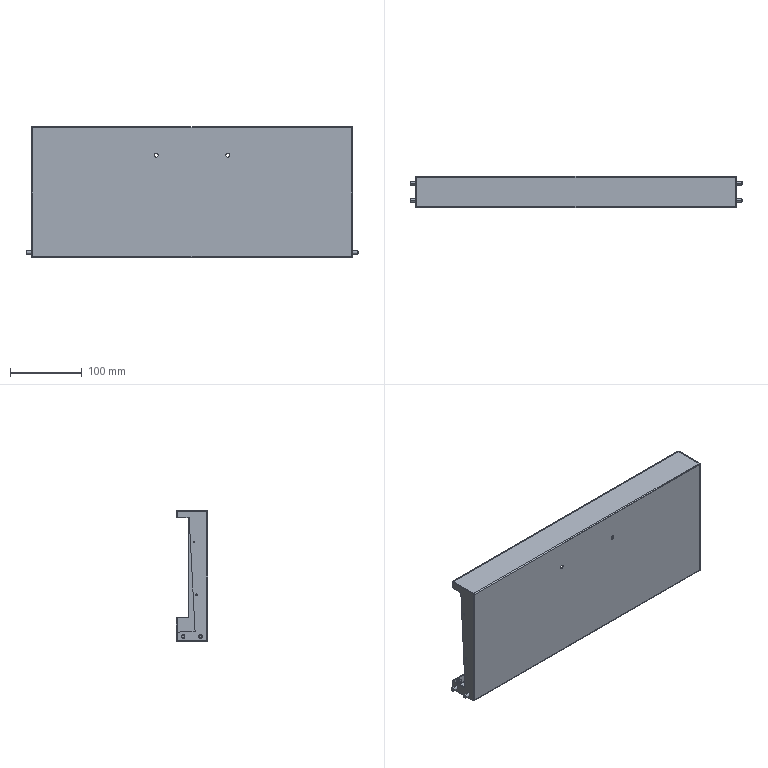Part | STEP file | 键盘盒-01^TY.NE-0002-01-014A 键盘盒-dddeger | 1 solid | 134 faces | box 464 x 43.4 x 183 mm | volume 167299 mm3 | plane 74 | cylinder 51 | torus 8 | spline 1 | commonest cylinder face diameters 2.8 x11 5 x8 0.4 x7 2 x4 2.5 x4 3.3 x4